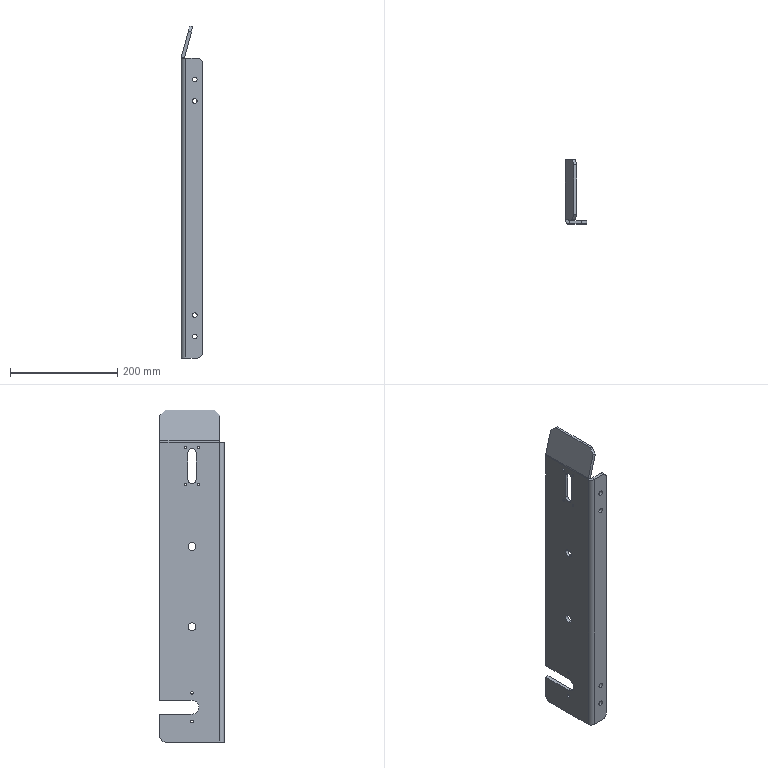Part | SolidWorks | features ICE 3, Fillet 2, HoleWzd 2, Chamfer 1, EdgeFlange 1, FlatPattern 1, SMBaseFlange 1, SheetMetal 1 | 1 solid | 60 faces | box 40 x 120 x 619.772 mm | volume 529398 mm3 | cylinder 35 | plane 25 | commonest cylinder face diameters 5 x12 9 x8 15 x7 20 x3 4 x2 16 x2